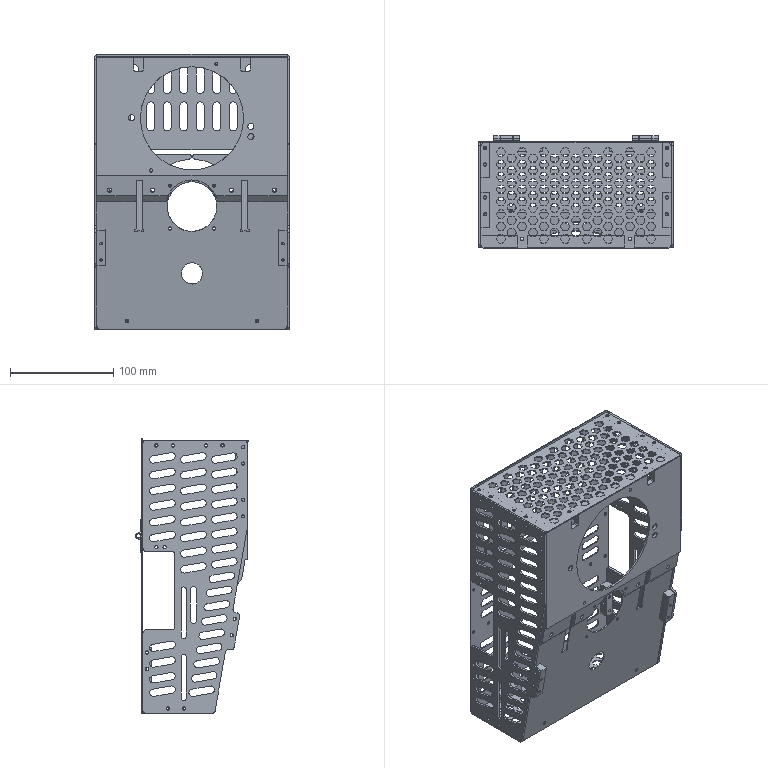Part | SolidWorks | 27 solids | 3616 faces | volume 253666 mm3 | cylinder 2054 | plane 1528 | spline 34 | commonest cylinder face diameters 3 x1197 7 x210 3.2 x200 2.5 x108 8 x100 6 x94